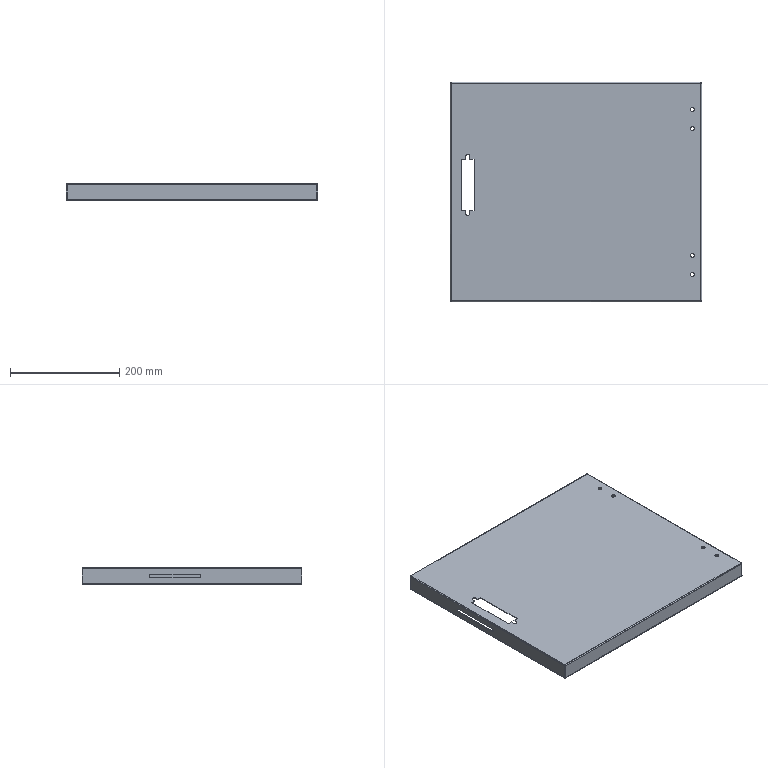Part | 1 solid | 95 faces | box 460 x 402 x 30 mm | volume 296686 mm3 | plane 50 | cylinder 29 | spline 16 | commonest cylinder face diameters 7 x13 1.473 x8 3.873 x8